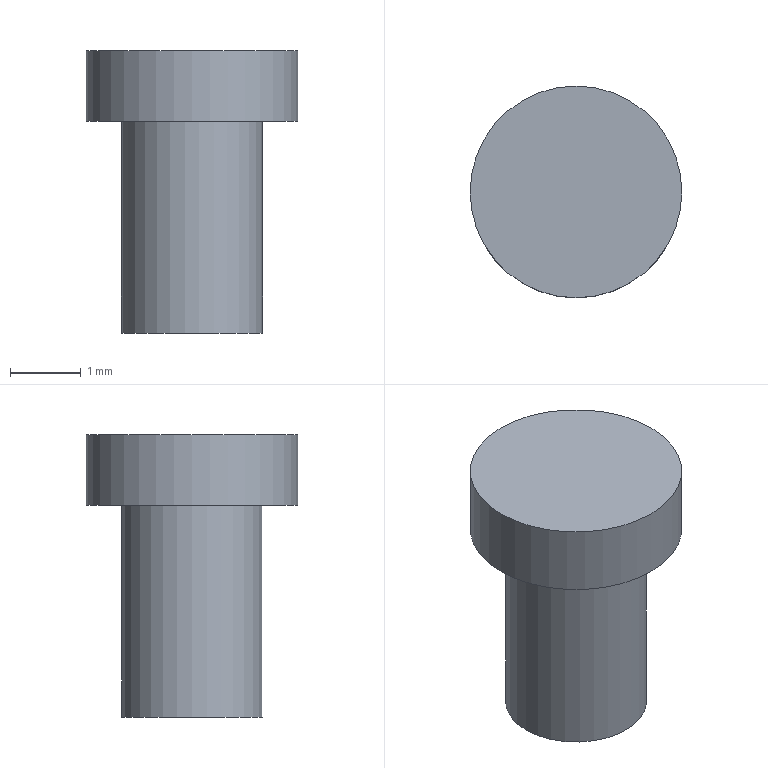Part | NX | features CYLINDER 2, DATUM_CSYS 1 | 1 solid | 5 faces | box 3 x 3 x 4 mm | volume 16.493 mm3 | plane 3 | cylinder 2 | commonest cylinder face diameters 2 x1 3 x1
STEP:
#1=CARTESIAN_POINT('',(1.,0.,0.));
#2=VERTEX_POINT('',#1);
#3=CARTESIAN_POINT('',(0.,0.,0.));
#4=DIRECTION('',(0.,0.,1.));
#5=DIRECTION('',(1.,0.,0.));
#6=AXIS2_PLACEMENT_3D('',#3,#4,#5);
#7=CIRCLE('',#6,1.);
#8=EDGE_CURVE('',#2,#2,#7,.T.);
#9=ORIENTED_EDGE('',*,*,#8,.F.);
#10=EDGE_LOOP('',(#9));
#11=FACE_BOUND('',#10,.T.);
#12=CARTESIAN_POINT('',(0.,0.,0.));
#13=DIRECTION('',(0.,0.,-1.));
#14=DIRECTION('',(-1.,0.,0.));
#15=AXIS2_PLACEMENT_3D('',#12,#13,#14);
#16=PLANE('',#15);
#17=ADVANCED_FACE('',(#11),#16,.T.);
#18=CARTESIAN_POINT('',(1.,0.,3.));
#19=VERTEX_POINT('',#18);
#20=CARTESIAN_POINT('',(0.,0.,3.));
#21=DIRECTION('',(0.,0.,-1.));
#22=DIRECTION('',(1.,0.,0.));
#23=AXIS2_PLACEMENT_3D('',#20,#21,#22);
#24=CIRCLE('',#23,1.);
#25=EDGE_CURVE('',#19,#19,#24,.T.);
#26=ORIENTED_EDGE('',*,*,#25,.T.);
#27=EDGE_LOOP('',(#26));
#28=FACE_BOUND('',#27,.T.);
#29=ORIENTED_EDGE('',*,*,#8,.T.);
#30=EDGE_LOOP('',(#29));
#31=FACE_BOUND('',#30,.T.);
#32=CARTESIAN_POINT('',(0.,0.,0.));
#33=DIRECTION('',(0.,0.,1.));
#34=DIRECTION('',(1.,0.,0.));
#35=AXIS2_PLACEMENT_3D('',#32,#33,#34);
#36=CYLINDRICAL_SURFACE('',#35,1.);
#37=ADVANCED_FACE('',(#28,#31),#36,.T.);
#38=CARTESIAN_POINT('',(1.5,0.,4.));
#39=VERTEX_POINT('',#38);
#40=CARTESIAN_POINT('',(0.,0.,4.));
#41=DIRECTION('',(0.,0.,-1.));
#42=DIRECTION('',(1.,0.,0.));
#43=AXIS2_PLACEMENT_3D('',#40,#41,#42);
#44=CIRCLE('',#43,1.5);
#45=EDGE_CURVE('',#39,#39,#44,.T.);
#46=ORIENTED_EDGE('',*,*,#45,.F.);
#47=EDGE_LOOP('',(#46));
#48=FACE_BOUND('',#47,.T.);
#49=CARTESIAN_POINT('',(0.,0.,4.));
#50=DIRECTION('',(0.,0.,1.));
#51=DIRECTION('',(1.,0.,0.));
#52=AXIS2_PLACEMENT_3D('',#49,#50,#51);
#53=PLANE('',#52);
#54=ADVANCED_FACE('',(#48),#53,.T.);
#55=ORIENTED_EDGE('',*,*,#25,.F.);
#56=EDGE_LOOP('',(#55));
#57=FACE_BOUND('',#56,.T.);
#58=CARTESIAN_POINT('',(1.5,0.,3.));
#59=VERTEX_POINT('',#58);
#60=CARTESIAN_POINT('',(0.,0.,3.));
#61=DIRECTION('',(0.,0.,1.));
#62=DIRECTION('',(1.,0.,0.));
#63=AXIS2_PLACEMENT_3D('',#60,#61,#62);
#64=CIRCLE('',#63,1.5);
#65=EDGE_CURVE('',#59,#59,#64,.T.);
#66=ORIENTED_EDGE('',*,*,#65,.F.);
#67=EDGE_LOOP('',(#66));
#68=FACE_BOUND('',#67,.T.);
#69=CARTESIAN_POINT('',(0.,0.,3.));
#70=DIRECTION('',(0.,0.,-1.));
#71=DIRECTION('',(-1.,0.,0.));
#72=AXIS2_PLACEMENT_3D('',#69,#70,#71);
#73=PLANE('',#72);
#74=ADVANCED_FACE('',(#57,#68),#73,.T.);
#75=ORIENTED_EDGE('',*,*,#45,.T.);
#76=EDGE_LOOP('',(#75));
#77=FACE_BOUND('',#76,.T.);
#78=ORIENTED_EDGE('',*,*,#65,.T.);
#79=EDGE_LOOP('',(#78));
#80=FACE_BOUND('',#79,.T.);
#81=CARTESIAN_POINT('',(0.,0.,3.));
#82=DIRECTION('',(0.,0.,1.));
#83=DIRECTION('',(1.,0.,0.));
#84=AXIS2_PLACEMENT_3D('',#81,#82,#83);
#85=CYLINDRICAL_SURFACE('',#84,1.5);
#86=ADVANCED_FACE('',(#77,#80),#85,.T.);
#87=CLOSED_SHELL('',(#17,#37,#54,#74,#86));
#88=MANIFOLD_SOLID_BREP('',#87);
#89=(LENGTH_UNIT()NAMED_UNIT(*)SI_UNIT(.MILLI.,.METRE.));
#90=UNCERTAINTY_MEASURE_WITH_UNIT(LENGTH_MEASURE(0.00001),#89,'','');
#91=(NAMED_UNIT(*)PLANE_ANGLE_UNIT()SI_UNIT($,.RADIAN.));
#92=(NAMED_UNIT(*)SI_UNIT($,.STERADIAN.)SOLID_ANGLE_UNIT());
#93=(GEOMETRIC_REPRESENTATION_CONTEXT(3)GLOBAL_UNCERTAINTY_ASSIGNED_CONTEXT((#90))GLOBAL_UNIT_ASSIGNED_CONTEXT((#89,#91,#92))REPRESENTATION_CONTEXT('',''));
#94=ADVANCED_BREP_SHAPE_REPRESENTATION('',(#88),#93);